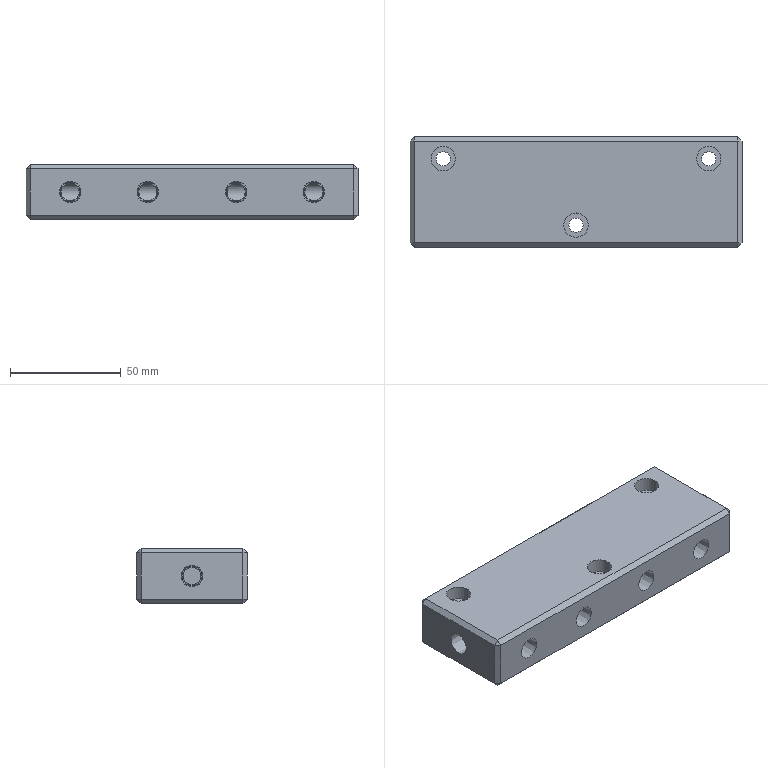Part | STEP file | P011002NM14-000 | 1 solid | 77 faces | box 150 x 50 x 25 mm | volume 168344 mm3 | plane 39 | cone 24 | cylinder 14 | commonest cylinder face diameters 8 x8 6.5 x3 11 x3